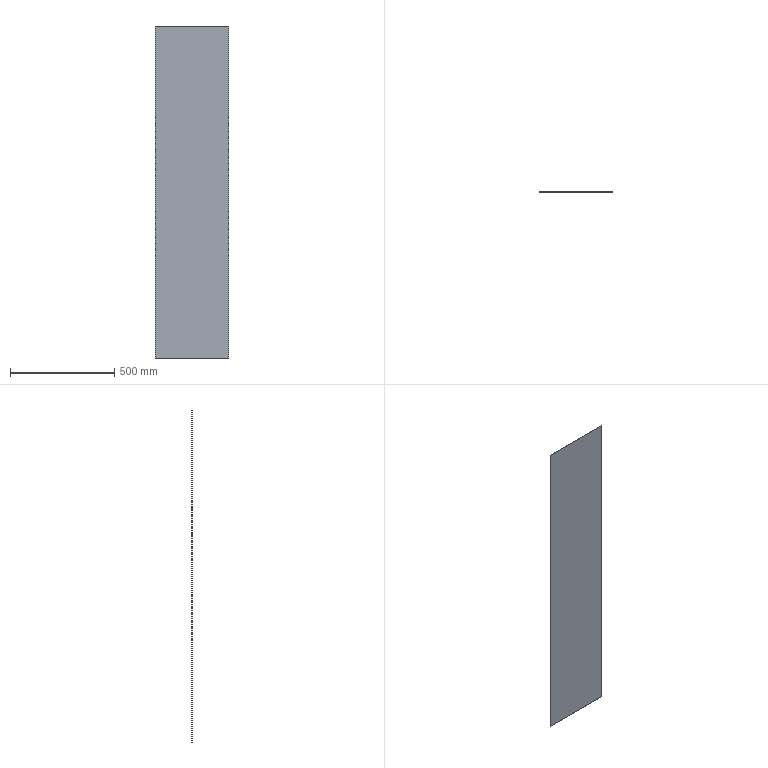Part | STEP file | Thin steel plate | 1 solid | 6 faces | box 350 x 1 x 1590 mm | volume 556500 mm3 | plane 6
STEP:
#1=CARTESIAN_POINT('',(318.149,16.377,1590.));
#2=VERTEX_POINT('',#1);
#3=CARTESIAN_POINT('',(318.149,16.377,0.));
#4=VERTEX_POINT('',#3);
#5=CARTESIAN_POINT('',(318.149,16.377,1590.));
#6=DIRECTION('',(0.,0.,-1.));
#7=VECTOR('',#6,1000.);
#8=LINE('',#5,#7);
#9=EDGE_CURVE('',#2,#4,#8,.T.);
#10=ORIENTED_EDGE('',*,*,#9,.F.);
#11=CARTESIAN_POINT('',(-31.851,16.377,1590.));
#12=VERTEX_POINT('',#11);
#13=CARTESIAN_POINT('',(-31.851,16.377,1590.));
#14=DIRECTION('',(1.,0.,0.));
#15=VECTOR('',#14,1000.);
#16=LINE('',#13,#15);
#17=EDGE_CURVE('',#12,#2,#16,.T.);
#18=ORIENTED_EDGE('',*,*,#17,.F.);
#19=CARTESIAN_POINT('',(-31.851,16.377,0.));
#20=VERTEX_POINT('',#19);
#21=CARTESIAN_POINT('',(-31.851,16.377,1590.));
#22=DIRECTION('',(0.,0.,1.));
#23=VECTOR('',#22,1000.);
#24=LINE('',#21,#23);
#25=EDGE_CURVE('',#20,#12,#24,.T.);
#26=ORIENTED_EDGE('',*,*,#25,.F.);
#27=CARTESIAN_POINT('',(-31.851,16.377,0.));
#28=DIRECTION('',(-1.,0.,0.));
#29=VECTOR('',#28,1000.);
#30=LINE('',#27,#29);
#31=EDGE_CURVE('',#4,#20,#30,.T.);
#32=ORIENTED_EDGE('',*,*,#31,.F.);
#33=EDGE_LOOP('',(#10,#18,#26,#32));
#34=FACE_OUTER_BOUND('',#33,.T.);
#35=CARTESIAN_POINT('',(-31.851,16.377,1590.));
#36=DIRECTION('',(0.,1.,0.));
#37=DIRECTION('',(0.,0.,1.));
#38=AXIS2_PLACEMENT_3D('',#35,#36,#37);
#39=PLANE('',#38);
#40=ADVANCED_FACE('',(#34),#39,.F.);
#41=CARTESIAN_POINT('',(318.149,17.377,0.));
#42=VERTEX_POINT('',#41);
#43=CARTESIAN_POINT('',(-31.851,17.377,0.));
#44=VERTEX_POINT('',#43);
#45=CARTESIAN_POINT('',(-31.851,17.377,0.));
#46=DIRECTION('',(-1.,0.,0.));
#47=VECTOR('',#46,1000.);
#48=LINE('',#45,#47);
#49=EDGE_CURVE('',#42,#44,#48,.T.);
#50=ORIENTED_EDGE('',*,*,#49,.F.);
#51=CARTESIAN_POINT('',(318.149,16.377,0.));
#52=DIRECTION('',(0.,1.,0.));
#53=VECTOR('',#52,1000.);
#54=LINE('',#51,#53);
#55=EDGE_CURVE('',#4,#42,#54,.T.);
#56=ORIENTED_EDGE('',*,*,#55,.F.);
#57=ORIENTED_EDGE('',*,*,#31,.T.);
#58=CARTESIAN_POINT('',(-31.851,16.377,0.));
#59=DIRECTION('',(0.,-1.,0.));
#60=VECTOR('',#59,1000.);
#61=LINE('',#58,#60);
#62=EDGE_CURVE('',#44,#20,#61,.T.);
#63=ORIENTED_EDGE('',*,*,#62,.F.);
#64=EDGE_LOOP('',(#50,#56,#57,#63));
#65=FACE_OUTER_BOUND('',#64,.T.);
#66=CARTESIAN_POINT('',(-31.851,16.377,0.));
#67=DIRECTION('',(0.,0.,1.));
#68=DIRECTION('',(1.,0.,0.));
#69=AXIS2_PLACEMENT_3D('',#66,#67,#68);
#70=PLANE('',#69);
#71=ADVANCED_FACE('',(#65),#70,.F.);
#72=CARTESIAN_POINT('',(318.149,17.377,1590.));
#73=VERTEX_POINT('',#72);
#74=CARTESIAN_POINT('',(318.149,17.377,1590.));
#75=DIRECTION('',(0.,0.,-1.));
#76=VECTOR('',#75,1000.);
#77=LINE('',#74,#76);
#78=EDGE_CURVE('',#73,#42,#77,.T.);
#79=ORIENTED_EDGE('',*,*,#78,.F.);
#80=CARTESIAN_POINT('',(318.149,17.377,1590.));
#81=DIRECTION('',(0.,1.,0.));
#82=VECTOR('',#81,1000.);
#83=LINE('',#80,#82);
#84=EDGE_CURVE('',#2,#73,#83,.T.);
#85=ORIENTED_EDGE('',*,*,#84,.F.);
#86=ORIENTED_EDGE('',*,*,#9,.T.);
#87=ORIENTED_EDGE('',*,*,#55,.T.);
#88=EDGE_LOOP('',(#79,#85,#86,#87));
#89=FACE_OUTER_BOUND('',#88,.T.);
#90=CARTESIAN_POINT('',(318.149,17.377,1590.));
#91=DIRECTION('',(-1.,0.,0.));
#92=DIRECTION('',(0.,0.,1.));
#93=AXIS2_PLACEMENT_3D('',#90,#91,#92);
#94=PLANE('',#93);
#95=ADVANCED_FACE('',(#89),#94,.F.);
#96=ORIENTED_EDGE('',*,*,#84,.T.);
#97=CARTESIAN_POINT('',(-31.851,17.377,1590.));
#98=VERTEX_POINT('',#97);
#99=CARTESIAN_POINT('',(-31.851,17.377,1590.));
#100=DIRECTION('',(-1.,0.,0.));
#101=VECTOR('',#100,1000.);
#102=LINE('',#99,#101);
#103=EDGE_CURVE('',#73,#98,#102,.T.);
#104=ORIENTED_EDGE('',*,*,#103,.T.);
#105=CARTESIAN_POINT('',(-31.851,16.377,1590.));
#106=DIRECTION('',(0.,-1.,0.));
#107=VECTOR('',#106,1000.);
#108=LINE('',#105,#107);
#109=EDGE_CURVE('',#98,#12,#108,.T.);
#110=ORIENTED_EDGE('',*,*,#109,.T.);
#111=ORIENTED_EDGE('',*,*,#17,.T.);
#112=EDGE_LOOP('',(#96,#104,#110,#111));
#113=FACE_OUTER_BOUND('',#112,.T.);
#114=CARTESIAN_POINT('',(-31.851,16.377,1590.));
#115=DIRECTION('',(0.,0.,1.));
#116=DIRECTION('',(1.,0.,0.));
#117=AXIS2_PLACEMENT_3D('',#114,#115,#116);
#118=PLANE('',#117);
#119=ADVANCED_FACE('',(#113),#118,.T.);
#120=ORIENTED_EDGE('',*,*,#25,.T.);
#121=ORIENTED_EDGE('',*,*,#109,.F.);
#122=CARTESIAN_POINT('',(-31.851,17.377,1590.));
#123=DIRECTION('',(0.,0.,1.));
#124=VECTOR('',#123,1000.);
#125=LINE('',#122,#124);
#126=EDGE_CURVE('',#44,#98,#125,.T.);
#127=ORIENTED_EDGE('',*,*,#126,.F.);
#128=ORIENTED_EDGE('',*,*,#62,.T.);
#129=EDGE_LOOP('',(#120,#121,#127,#128));
#130=FACE_OUTER_BOUND('',#129,.T.);
#131=CARTESIAN_POINT('',(-31.851,17.377,1590.));
#132=DIRECTION('',(1.,0.,0.));
#133=DIRECTION('',(0.,0.,-1.));
#134=AXIS2_PLACEMENT_3D('',#131,#132,#133);
#135=PLANE('',#134);
#136=ADVANCED_FACE('',(#130),#135,.F.);
#137=ORIENTED_EDGE('',*,*,#126,.T.);
#138=ORIENTED_EDGE('',*,*,#103,.F.);
#139=ORIENTED_EDGE('',*,*,#78,.T.);
#140=ORIENTED_EDGE('',*,*,#49,.T.);
#141=EDGE_LOOP('',(#137,#138,#139,#140));
#142=FACE_OUTER_BOUND('',#141,.T.);
#143=CARTESIAN_POINT('',(-31.851,17.377,1590.));
#144=DIRECTION('',(0.,-1.,0.));
#145=DIRECTION('',(0.,0.,-1.));
#146=AXIS2_PLACEMENT_3D('',#143,#144,#145);
#147=PLANE('',#146);
#148=ADVANCED_FACE('',(#142),#147,.F.);
#149=CLOSED_SHELL('',(#40,#71,#95,#119,#136,#148));
#150=MANIFOLD_SOLID_BREP('',#149);
#151=CARTESIAN_POINT('',(0.,0.,0.));
#152=DIRECTION('',(0.,0.,1.));
#153=DIRECTION('',(1.,0.,0.));
#154=AXIS2_PLACEMENT_3D('',#151,#152,#153);
#155=(LENGTH_UNIT()NAMED_UNIT(*)SI_UNIT(.MILLI.,.METRE.));
#156=UNCERTAINTY_MEASURE_WITH_UNIT(LENGTH_MEASURE(0.00001),#155,'','');
#157=(NAMED_UNIT(*)PLANE_ANGLE_UNIT()SI_UNIT($,.RADIAN.));
#158=(NAMED_UNIT(*)SI_UNIT($,.STERADIAN.)SOLID_ANGLE_UNIT());
#159=(GEOMETRIC_REPRESENTATION_CONTEXT(3)GLOBAL_UNCERTAINTY_ASSIGNED_CONTEXT((#156))GLOBAL_UNIT_ASSIGNED_CONTEXT((#155,#157,#158))REPRESENTATION_CONTEXT('',''));
#160=ADVANCED_BREP_SHAPE_REPRESENTATION('',(#150,#154),#159);